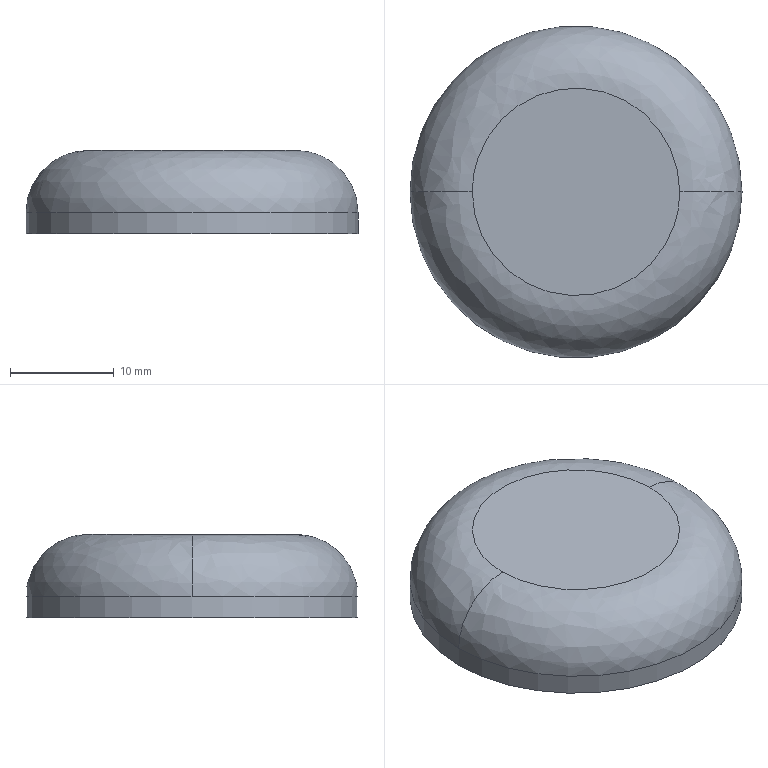Part | STEP file | 5091207W | 1 solid | 5 faces | box 32 x 32 x 8 mm | volume 5722 mm3 | plane 2 | spline 2 | cylinder 1 | commonest cylinder face diameters 32 x1
STEP:
#1=CARTESIAN_POINT('',(0.,0.,0.));
#2=DIRECTION('',(0.,0.,1.));
#3=DIRECTION('',(1.,0.,0.));
#4=AXIS2_PLACEMENT_3D('',#1,#2,#3);
#5=CARTESIAN_POINT('',(16.,-88.,34.));
#6=VERTEX_POINT('',#5);
#7=CARTESIAN_POINT('',(0.,-88.,34.));
#8=DIRECTION('',(0.,0.,1.));
#9=DIRECTION('',(1.,0.,0.));
#10=AXIS2_PLACEMENT_3D('',#7,#8,#9);
#11=CIRCLE('',#10,16.);
#12=CARTESIAN_POINT('',(16.64,-71.349,34.));
#13=DIRECTION('',(0.,0.,1.));
#14=DIRECTION('',(-1.,0.,0.));
#15=AXIS2_PLACEMENT_3D('',#12,#13,#14);
#16=PLANE('',#15);
#17=CARTESIAN_POINT('',(16.64,16.651));
#18=DIRECTION('',(-1.,0.));
#19=AXIS2_PLACEMENT_2D('',#17,#18);
#20=CIRCLE('',#19,16.);
#21=(GEOMETRIC_REPRESENTATION_CONTEXT(2)PARAMETRIC_REPRESENTATION_CONTEXT()REPRESENTATION_CONTEXT('',''));
#22=DEFINITIONAL_REPRESENTATION('',(#20),#21);
#23=PCURVE('',#16,#22);
#24=CARTESIAN_POINT('',(0.,-88.,34.));
#25=DIRECTION('',(0.,0.,1.));
#26=DIRECTION('',(1.,0.,0.));
#27=AXIS2_PLACEMENT_3D('',#24,#25,#26);
#28=CYLINDRICAL_SURFACE('',#27,16.);
#29=CARTESIAN_POINT('',(0.,0.));
#30=DIRECTION('',(1.,0.));
#31=VECTOR('',#30,1.);
#32=LINE('',#29,#31);
#33=(GEOMETRIC_REPRESENTATION_CONTEXT(2)PARAMETRIC_REPRESENTATION_CONTEXT()REPRESENTATION_CONTEXT('',''));
#34=DEFINITIONAL_REPRESENTATION('',(#32),#33);
#35=PCURVE('',#28,#34);
#36=SURFACE_CURVE('',#11,(#23,#35),.PCURVE_S1.);
#37=EDGE_CURVE('',#6,#6,#36,.T.);
#38=ORIENTED_EDGE('',*,*,#37,.F.);
#39=EDGE_LOOP('',(#38));
#40=FACE_BOUND('',#39,.T.);
#41=ADVANCED_FACE('',(#40),#16,.F.);
#42=ORIENTED_EDGE('',*,*,#37,.T.);
#43=CARTESIAN_POINT('',(16.,-88.,36.));
#44=VERTEX_POINT('',#43);
#45=CARTESIAN_POINT('',(16.,-88.,34.));
#46=CARTESIAN_POINT('',(16.,-88.,36.));
#47=B_SPLINE_CURVE_WITH_KNOTS('',1,(#45,#46),.UNSPECIFIED.,.F.,.F.,(2,2),(0.,2.),.PIECEWISE_BEZIER_KNOTS.);
#48=CARTESIAN_POINT('',(6.283,0.));
#49=DIRECTION('',(0.,1.));
#50=VECTOR('',#49,1.);
#51=LINE('',#48,#50);
#52=(GEOMETRIC_REPRESENTATION_CONTEXT(2)PARAMETRIC_REPRESENTATION_CONTEXT()REPRESENTATION_CONTEXT('',''));
#53=DEFINITIONAL_REPRESENTATION('',(#51),#52);
#54=PCURVE('',#28,#53);
#55=CARTESIAN_POINT('',(0.,0.));
#56=DIRECTION('',(0.,1.));
#57=VECTOR('',#56,1.);
#58=LINE('',#55,#57);
#59=(GEOMETRIC_REPRESENTATION_CONTEXT(2)PARAMETRIC_REPRESENTATION_CONTEXT()REPRESENTATION_CONTEXT('',''));
#60=DEFINITIONAL_REPRESENTATION('',(#58),#59);
#61=PCURVE('',#28,#60);
#62=SEAM_CURVE('',#47,(#54,#61),.PCURVE_S1.);
#63=EDGE_CURVE('',#6,#44,#62,.T.);
#64=ORIENTED_EDGE('',*,*,#63,.T.);
#65=CARTESIAN_POINT('',(-16.,-88.,36.));
#66=VERTEX_POINT('',#65);
#67=CARTESIAN_POINT('',(0.,-88.,36.));
#68=DIRECTION('',(0.,0.,1.));
#69=DIRECTION('',(-1.,0.,0.));
#70=AXIS2_PLACEMENT_3D('',#67,#68,#69);
#71=CIRCLE('',#70,16.);
#72=CARTESIAN_POINT('',(3.142,2.));
#73=DIRECTION('',(1.,0.));
#74=VECTOR('',#73,1.);
#75=LINE('',#72,#74);
#76=(GEOMETRIC_REPRESENTATION_CONTEXT(2)PARAMETRIC_REPRESENTATION_CONTEXT()REPRESENTATION_CONTEXT('',''));
#77=DEFINITIONAL_REPRESENTATION('',(#75),#76);
#78=PCURVE('',#28,#77);
#79=CARTESIAN_POINT('',(-16.,-88.,36.));
#80=CARTESIAN_POINT('',(-16.,-120.,36.));
#81=CARTESIAN_POINT('',(16.,-120.,36.));
#82=CARTESIAN_POINT('',(16.,-88.,36.));
#83=CARTESIAN_POINT('',(-16.,-88.,39.541));
#84=CARTESIAN_POINT('',(-16.,-120.,39.541));
#85=CARTESIAN_POINT('',(16.,-120.,39.541));
#86=CARTESIAN_POINT('',(16.,-88.,39.541));
#87=CARTESIAN_POINT('',(-13.485,-88.,42.03));
#88=CARTESIAN_POINT('',(-13.485,-114.97,42.03));
#89=CARTESIAN_POINT('',(13.485,-114.97,42.03));
#90=CARTESIAN_POINT('',(13.485,-88.,42.03));
#91=CARTESIAN_POINT('',(-9.949,-88.,42.));
#92=CARTESIAN_POINT('',(-9.949,-107.898,42.));
#93=CARTESIAN_POINT('',(9.949,-107.898,42.));
#94=CARTESIAN_POINT('',(9.949,-88.,42.));
#95=(BOUNDED_SURFACE()B_SPLINE_SURFACE(3,3,((#79,#80,#81,#82),(#83,#84,#85,#86),(#87,#88,#89,#90),(#91,#92,#93,#94)),.UNSPECIFIED.,.F.,.F.,.F.)B_SPLINE_SURFACE_WITH_KNOTS((4,4),(4,4),(0.0214,0.9843),(0.,1.),.PIECEWISE_BEZIER_KNOTS.)GEOMETRIC_REPRESENTATION_ITEM()RATIONAL_B_SPLINE_SURFACE(((0.9868,0.3289,0.3289,0.9868),(0.7929,0.2643,0.2643,0.7929),(0.7941,0.2647,0.2647,0.7941),(0.9903,0.3301,0.3301,0.9903)))REPRESENTATION_ITEM('')SURFACE());
#96=CARTESIAN_POINT('',(0.0214,0.));
#97=CARTESIAN_POINT('',(0.0214,0.02375));
#98=CARTESIAN_POINT('',(0.0214,0.06805));
#99=CARTESIAN_POINT('',(0.0214,0.1267));
#100=CARTESIAN_POINT('',(0.0214,0.1794));
#101=CARTESIAN_POINT('',(0.0214,0.2276));
#102=CARTESIAN_POINT('',(0.0214,0.2721));
#103=CARTESIAN_POINT('',(0.0214,0.3139));
#104=CARTESIAN_POINT('',(0.0214,0.3535));
#105=CARTESIAN_POINT('',(0.0214,0.3914));
#106=CARTESIAN_POINT('',(0.0214,0.4282));
#107=CARTESIAN_POINT('',(0.0214,0.4643));
#108=CARTESIAN_POINT('',(0.0214,0.5));
#109=CARTESIAN_POINT('',(0.0214,0.5357));
#110=CARTESIAN_POINT('',(0.0214,0.5718));
#111=CARTESIAN_POINT('',(0.0214,0.6086));
#112=CARTESIAN_POINT('',(0.0214,0.6465));
#113=CARTESIAN_POINT('',(0.0214,0.6861));
#114=CARTESIAN_POINT('',(0.0214,0.7279));
#115=CARTESIAN_POINT('',(0.0214,0.7724));
#116=CARTESIAN_POINT('',(0.0214,0.8206));
#117=CARTESIAN_POINT('',(0.0214,0.8733));
#118=CARTESIAN_POINT('',(0.0214,0.9319));
#119=CARTESIAN_POINT('',(0.0214,0.9763));
#120=CARTESIAN_POINT('',(0.0214,1.));
#121=B_SPLINE_CURVE_WITH_KNOTS('',3,(#96,#97,#98,#99,#100,#101,#102,#103,#104,#105,#106,#107,#108,#109,#110,#111,#112,#113,#114,#115,#116,#117,#118,#119,#120),.UNSPECIFIED.,.F.,.F.,(4,1,1,1,1,1,1,1,1,1,1,1,1,1,1,1,1,1,1,1,1,1,4),(0.,0.1428,0.2856,0.4284,0.5712,0.714,0.8568,0.9996,1.142,1.285,1.428,1.571,1.714,1.856,1.999,2.142,2.285,2.428,2.57,2.713,2.856,2.999,3.142),.QUASI_UNIFORM_KNOTS.);
#122=(GEOMETRIC_REPRESENTATION_CONTEXT(2)PARAMETRIC_REPRESENTATION_CONTEXT()REPRESENTATION_CONTEXT('',''));
#123=DEFINITIONAL_REPRESENTATION('',(#121),#122);
#124=PCURVE('',#95,#123);
#125=SURFACE_CURVE('',#71,(#78,#124),.PCURVE_S1.);
#126=EDGE_CURVE('',#66,#44,#125,.T.);
#127=ORIENTED_EDGE('',*,*,#126,.F.);
#128=CARTESIAN_POINT('',(0.,-88.,36.));
#129=DIRECTION('',(0.,0.,1.));
#130=DIRECTION('',(-1.,0.,0.));
#131=AXIS2_PLACEMENT_3D('',#128,#129,#130);
#132=CIRCLE('',#131,16.);
#133=CARTESIAN_POINT('',(-3.142,2.));
#134=DIRECTION('',(1.,0.));
#135=VECTOR('',#134,1.);
#136=LINE('',#133,#135);
#137=(GEOMETRIC_REPRESENTATION_CONTEXT(2)PARAMETRIC_REPRESENTATION_CONTEXT()REPRESENTATION_CONTEXT('',''));
#138=DEFINITIONAL_REPRESENTATION('',(#136),#137);
#139=PCURVE('',#28,#138);
#140=CARTESIAN_POINT('',(16.,-88.,36.));
#141=CARTESIAN_POINT('',(16.,-56.,36.));
#142=CARTESIAN_POINT('',(-16.,-56.,36.));
#143=CARTESIAN_POINT('',(-16.,-88.,36.));
#144=CARTESIAN_POINT('',(16.,-88.,39.541));
#145=CARTESIAN_POINT('',(16.,-56.,39.541));
#146=CARTESIAN_POINT('',(-16.,-56.,39.541));
#147=CARTESIAN_POINT('',(-16.,-88.,39.541));
#148=CARTESIAN_POINT('',(13.485,-88.,42.03));
#149=CARTESIAN_POINT('',(13.485,-61.03,42.03));
#150=CARTESIAN_POINT('',(-13.485,-61.03,42.03));
#151=CARTESIAN_POINT('',(-13.485,-88.,42.03));
#152=CARTESIAN_POINT('',(9.949,-88.,42.));
#153=CARTESIAN_POINT('',(9.949,-68.102,42.));
#154=CARTESIAN_POINT('',(-9.949,-68.102,42.));
#155=CARTESIAN_POINT('',(-9.949,-88.,42.));
#156=(BOUNDED_SURFACE()B_SPLINE_SURFACE(3,3,((#140,#141,#142,#143),(#144,#145,#146,#147),(#148,#149,#150,#151),(#152,#153,#154,#155)),.UNSPECIFIED.,.F.,.F.,.F.)B_SPLINE_SURFACE_WITH_KNOTS((4,4),(4,4),(0.0214,0.9843),(0.,1.),.PIECEWISE_BEZIER_KNOTS.)GEOMETRIC_REPRESENTATION_ITEM()RATIONAL_B_SPLINE_SURFACE(((0.9868,0.3289,0.3289,0.9868),(0.7929,0.2643,0.2643,0.7929),(0.7941,0.2647,0.2647,0.7941),(0.9903,0.3301,0.3301,0.9903)))REPRESENTATION_ITEM('')SURFACE());
#157=CARTESIAN_POINT('',(0.0214,0.));
#158=CARTESIAN_POINT('',(0.0214,0.02375));
#159=CARTESIAN_POINT('',(0.0214,0.06805));
#160=CARTESIAN_POINT('',(0.0214,0.1267));
#161=CARTESIAN_POINT('',(0.0214,0.1794));
#162=CARTESIAN_POINT('',(0.0214,0.2276));
#163=CARTESIAN_POINT('',(0.0214,0.2721));
#164=CARTESIAN_POINT('',(0.0214,0.3139));
#165=CARTESIAN_POINT('',(0.0214,0.3535));
#166=CARTESIAN_POINT('',(0.0214,0.3914));
#167=CARTESIAN_POINT('',(0.0214,0.4282));
#168=CARTESIAN_POINT('',(0.0214,0.4643));
#169=CARTESIAN_POINT('',(0.0214,0.5));
#170=CARTESIAN_POINT('',(0.0214,0.5357));
#171=CARTESIAN_POINT('',(0.0214,0.5718));
#172=CARTESIAN_POINT('',(0.0214,0.6086));
#173=CARTESIAN_POINT('',(0.0214,0.6465));
#174=CARTESIAN_POINT('',(0.0214,0.6861));
#175=CARTESIAN_POINT('',(0.0214,0.7279));
#176=CARTESIAN_POINT('',(0.0214,0.7724));
#177=CARTESIAN_POINT('',(0.0214,0.8206));
#178=CARTESIAN_POINT('',(0.0214,0.8733));
#179=CARTESIAN_POINT('',(0.0214,0.9319));
#180=CARTESIAN_POINT('',(0.0214,0.9763));
#181=CARTESIAN_POINT('',(0.0214,1.));
#182=B_SPLINE_CURVE_WITH_KNOTS('',3,(#157,#158,#159,#160,#161,#162,#163,#164,#165,#166,#167,#168,#169,#170,#171,#172,#173,#174,#175,#176,#177,#178,#179,#180,#181),.UNSPECIFIED.,.F.,.F.,(4,1,1,1,1,1,1,1,1,1,1,1,1,1,1,1,1,1,1,1,1,1,4),(3.142,3.284,3.427,3.57,3.713,3.856,3.998,4.141,4.284,4.427,4.57,4.712,4.855,4.998,5.141,5.284,5.426,5.569,5.712,5.855,5.998,6.14,6.283),.QUASI_UNIFORM_KNOTS.);
#183=(GEOMETRIC_REPRESENTATION_CONTEXT(2)PARAMETRIC_REPRESENTATION_CONTEXT()REPRESENTATION_CONTEXT('',''));
#184=DEFINITIONAL_REPRESENTATION('',(#182),#183);
#185=PCURVE('',#156,#184);
#186=SURFACE_CURVE('',#132,(#139,#185),.PCURVE_S1.);
#187=EDGE_CURVE('',#44,#66,#186,.T.);
#188=ORIENTED_EDGE('',*,*,#187,.F.);
#189=ORIENTED_EDGE('',*,*,#63,.F.);
#190=EDGE_LOOP('',(#42,#64,#127,#188,#189));
#191=FACE_BOUND('',#190,.T.);
#192=ADVANCED_FACE('',(#191),#28,.T.);
#193=CARTESIAN_POINT('',(10.,-88.,42.));
#194=VERTEX_POINT('',#193);
#195=CARTESIAN_POINT('',(10.,-88.,36.));
#196=DIRECTION('',(0.,-1.,0.));
#197=DIRECTION('',(1.,0.,0.));
#198=AXIS2_PLACEMENT_3D('',#195,#196,#197);
#199=CIRCLE('',#198,6.);
#200=CARTESIAN_POINT('',(0.0214,0.));
#201=CARTESIAN_POINT('',(0.03751,0.));
#202=CARTESIAN_POINT('',(0.06926,0.));
#203=CARTESIAN_POINT('',(0.1156,0.));
#204=CARTESIAN_POINT('',(0.1609,0.));
#205=CARTESIAN_POINT('',(0.2052,0.));
#206=CARTESIAN_POINT('',(0.2488,0.));
#207=CARTESIAN_POINT('',(0.2916,0.));
#208=CARTESIAN_POINT('',(0.3339,0.));
#209=CARTESIAN_POINT('',(0.3758,0.));
#210=CARTESIAN_POINT('',(0.4174,0.));
#211=CARTESIAN_POINT('',(0.4588,0.));
#212=CARTESIAN_POINT('',(0.5,0.));
#213=CARTESIAN_POINT('',(0.5412,0.));
#214=CARTESIAN_POINT('',(0.5826,0.));
#215=CARTESIAN_POINT('',(0.6242,0.));
#216=CARTESIAN_POINT('',(0.6661,0.));
#217=CARTESIAN_POINT('',(0.7084,0.));
#218=CARTESIAN_POINT('',(0.7512,0.));
#219=CARTESIAN_POINT('',(0.7948,0.));
#220=CARTESIAN_POINT('',(0.8391,0.));
#221=CARTESIAN_POINT('',(0.8844,0.));
#222=CARTESIAN_POINT('',(0.9307,0.));
#223=CARTESIAN_POINT('',(0.9625,0.));
#224=CARTESIAN_POINT('',(0.9786,0.));
#225=B_SPLINE_CURVE_WITH_KNOTS('',3,(#200,#201,#202,#203,#204,#205,#206,#207,#208,#209,#210,#211,#212,#213,#214,#215,#216,#217,#218,#219,#220,#221,#222,#223,#224),.UNSPECIFIED.,.F.,.F.,(4,1,1,1,1,1,1,1,1,1,1,1,1,1,1,1,1,1,1,1,1,1,4),(0.,0.0714,0.1428,0.2142,0.2856,0.357,0.4284,0.4998,0.5712,0.6426,0.714,0.7854,0.8568,0.9282,0.9996,1.071,1.142,1.214,1.285,1.357,1.428,1.499,1.571),.QUASI_UNIFORM_KNOTS.);
#226=(GEOMETRIC_REPRESENTATION_CONTEXT(2)PARAMETRIC_REPRESENTATION_CONTEXT()REPRESENTATION_CONTEXT('',''));
#227=DEFINITIONAL_REPRESENTATION('',(#225),#226);
#228=PCURVE('',#156,#227);
#229=CARTESIAN_POINT('',(0.0214,1.));
#230=CARTESIAN_POINT('',(0.03751,1.));
#231=CARTESIAN_POINT('',(0.06926,1.));
#232=CARTESIAN_POINT('',(0.1156,1.));
#233=CARTESIAN_POINT('',(0.1609,1.));
#234=CARTESIAN_POINT('',(0.2052,1.));
#235=CARTESIAN_POINT('',(0.2488,1.));
#236=CARTESIAN_POINT('',(0.2916,1.));
#237=CARTESIAN_POINT('',(0.3339,1.));
#238=CARTESIAN_POINT('',(0.3758,1.));
#239=CARTESIAN_POINT('',(0.4174,1.));
#240=CARTESIAN_POINT('',(0.4588,1.));
#241=CARTESIAN_POINT('',(0.5,1.));
#242=CARTESIAN_POINT('',(0.5412,1.));
#243=CARTESIAN_POINT('',(0.5826,1.));
#244=CARTESIAN_POINT('',(0.6242,1.));
#245=CARTESIAN_POINT('',(0.6661,1.));
#246=CARTESIAN_POINT('',(0.7084,1.));
#247=CARTESIAN_POINT('',(0.7512,1.));
#248=CARTESIAN_POINT('',(0.7948,1.));
#249=CARTESIAN_POINT('',(0.8391,1.));
#250=CARTESIAN_POINT('',(0.8844,1.));
#251=CARTESIAN_POINT('',(0.9307,1.));
#252=CARTESIAN_POINT('',(0.9625,1.));
#253=CARTESIAN_POINT('',(0.9786,1.));
#254=B_SPLINE_CURVE_WITH_KNOTS('',3,(#229,#230,#231,#232,#233,#234,#235,#236,#237,#238,#239,#240,#241,#242,#243,#244,#245,#246,#247,#248,#249,#250,#251,#252,#253),.UNSPECIFIED.,.F.,.F.,(4,1,1,1,1,1,1,1,1,1,1,1,1,1,1,1,1,1,1,1,1,1,4),(0.,0.0714,0.1428,0.2142,0.2856,0.357,0.4284,0.4998,0.5712,0.6426,0.714,0.7854,0.8568,0.9282,0.9996,1.071,1.142,1.214,1.285,1.357,1.428,1.499,1.571),.QUASI_UNIFORM_KNOTS.);
#255=(GEOMETRIC_REPRESENTATION_CONTEXT(2)PARAMETRIC_REPRESENTATION_CONTEXT()REPRESENTATION_CONTEXT('',''));
#256=DEFINITIONAL_REPRESENTATION('',(#254),#255);
#257=PCURVE('',#95,#256);
#258=SURFACE_CURVE('',#199,(#228,#257),.PCURVE_S1.);
#259=EDGE_CURVE('',#44,#194,#258,.T.);
#260=ORIENTED_EDGE('',*,*,#259,.T.);
#261=CARTESIAN_POINT('',(-10.,-87.956,42.));
#262=VERTEX_POINT('',#261);
#263=CARTESIAN_POINT('',(10.,-88.,42.));
#264=CARTESIAN_POINT('',(10.,-87.344,42.));
#265=CARTESIAN_POINT('',(9.936,-86.695,42.));
#266=CARTESIAN_POINT('',(9.681,-85.409,42.));
#267=CARTESIAN_POINT('',(9.491,-84.784,42.));
#268=CARTESIAN_POINT('',(8.99,-83.573,42.));
#269=CARTESIAN_POINT('',(8.683,-82.996,42.));
#270=CARTESIAN_POINT('',(7.956,-81.906,42.));
#271=CARTESIAN_POINT('',(7.542,-81.401,42.));
#272=CARTESIAN_POINT('',(6.616,-80.473,42.));
#273=CARTESIAN_POINT('',(6.112,-80.058,42.));
#274=CARTESIAN_POINT('',(5.023,-79.328,42.));
#275=CARTESIAN_POINT('',(4.447,-79.019,42.));
#276=CARTESIAN_POINT('',(3.237,-78.516,42.));
#277=CARTESIAN_POINT('',(2.612,-78.325,42.));
#278=CARTESIAN_POINT('',(1.327,-78.067,42.));
#279=CARTESIAN_POINT('',(0.6774,-78.002,42.));
#280=CARTESIAN_POINT('',(-0.6332,-77.999,42.));
#281=CARTESIAN_POINT('',(-1.283,-78.061,42.));
#282=CARTESIAN_POINT('',(-2.57,-78.314,42.));
#283=CARTESIAN_POINT('',(-3.195,-78.502,42.));
#284=CARTESIAN_POINT('',(-4.407,-79.,42.));
#285=CARTESIAN_POINT('',(-4.984,-79.306,42.));
#286=CARTESIAN_POINT('',(-6.076,-80.031,42.));
#287=CARTESIAN_POINT('',(-6.583,-80.444,42.));
#288=CARTESIAN_POINT('',(-7.513,-81.367,42.));
#289=CARTESIAN_POINT('',(-7.929,-81.871,42.));
#290=CARTESIAN_POINT('',(-8.661,-82.958,42.));
#291=CARTESIAN_POINT('',(-8.971,-83.533,42.));
#292=CARTESIAN_POINT('',(-9.477,-84.742,42.));
#293=CARTESIAN_POINT('',(-9.669,-85.367,42.));
#294=CARTESIAN_POINT('',(-9.93,-86.651,42.));
#295=CARTESIAN_POINT('',(-9.997,-87.3,42.));
#296=CARTESIAN_POINT('',(-10.,-87.956,42.));
#297=B_SPLINE_CURVE_WITH_KNOTS('',3,(#263,#264,#265,#266,#267,#268,#269,#270,#271,#272,#273,#274,#275,#276,#277,#278,#279,#280,#281,#282,#283,#284,#285,#286,#287,#288,#289,#290,#291,#292,#293,#294,#295,#296),.UNSPECIFIED.,.F.,.F.,(4,2,2,2,2,2,2,2,2,2,2,2,2,2,2,2,4),(0.,0.0625,0.125,0.1875,0.25,0.3125,0.375,0.4375,0.5,0.5625,0.625,0.6875,0.75,0.8125,0.875,0.9375,1.),.UNSPECIFIED.);
#298=CARTESIAN_POINT('',(0.9786,0.));
#299=CARTESIAN_POINT('',(0.9786,0.007948));
#300=CARTESIAN_POINT('',(0.9786,0.02343));
#301=CARTESIAN_POINT('',(0.9786,0.04558));
#302=CARTESIAN_POINT('',(0.9786,0.06678));
#303=CARTESIAN_POINT('',(0.9786,0.08717));
#304=CARTESIAN_POINT('',(0.9786,0.1068));
#305=CARTESIAN_POINT('',(0.9786,0.1257));
#306=CARTESIAN_POINT('',(0.9786,0.1439));
#307=CARTESIAN_POINT('',(0.9786,0.1615));
#308=CARTESIAN_POINT('',(0.9786,0.1786));
#309=CARTESIAN_POINT('',(0.9786,0.1951));
#310=CARTESIAN_POINT('',(0.9786,0.2111));
#311=CARTESIAN_POINT('',(0.9786,0.2268));
#312=CARTESIAN_POINT('',(0.9786,0.242));
#313=CARTESIAN_POINT('',(0.9786,0.2569));
#314=CARTESIAN_POINT('',(0.9786,0.2714));
#315=CARTESIAN_POINT('',(0.9786,0.2856));
#316=CARTESIAN_POINT('',(0.9786,0.2996));
#317=CARTESIAN_POINT('',(0.9786,0.3132));
#318=CARTESIAN_POINT('',(0.9786,0.3266));
#319=CARTESIAN_POINT('',(0.9786,0.3398));
#320=CARTESIAN_POINT('',(0.9786,0.3529));
#321=CARTESIAN_POINT('',(0.9786,0.3657));
#322=CARTESIAN_POINT('',(0.9786,0.3783));
#323=CARTESIAN_POINT('',(0.9786,0.3908));
#324=CARTESIAN_POINT('',(0.9786,0.4032));
#325=CARTESIAN_POINT('',(0.9786,0.4155));
#326=CARTESIAN_POINT('',(0.9786,0.4277));
#327=CARTESIAN_POINT('',(0.9786,0.4397));
#328=CARTESIAN_POINT('',(0.9786,0.4518));
#329=CARTESIAN_POINT('',(0.9786,0.4638));
#330=CARTESIAN_POINT('',(0.9786,0.4757));
#331=CARTESIAN_POINT('',(0.9786,0.4875));
#332=CARTESIAN_POINT('',(0.9786,0.4994));
#333=CARTESIAN_POINT('',(0.9786,0.5113));
#334=CARTESIAN_POINT('',(0.9786,0.5232));
#335=CARTESIAN_POINT('',(0.9786,0.5351));
#336=CARTESIAN_POINT('',(0.9786,0.5471));
#337=CARTESIAN_POINT('',(0.9786,0.5591));
#338=CARTESIAN_POINT('',(0.9786,0.5712));
#339=CARTESIAN_POINT('',(0.9786,0.5834));
#340=CARTESIAN_POINT('',(0.9786,0.5956));
#341=CARTESIAN_POINT('',(0.9786,0.608));
#342=CARTESIAN_POINT('',(0.9786,0.6205));
#343=CARTESIAN_POINT('',(0.9786,0.6331));
#344=CARTESIAN_POINT('',(0.9786,0.6459));
#345=CARTESIAN_POINT('',(0.9786,0.659));
#346=CARTESIAN_POINT('',(0.9786,0.6721));
#347=CARTESIAN_POINT('',(0.9786,0.6855));
#348=CARTESIAN_POINT('',(0.9786,0.6992));
#349=CARTESIAN_POINT('',(0.9786,0.7131));
#350=CARTESIAN_POINT('',(0.9786,0.7273));
#351=CARTESIAN_POINT('',(0.9786,0.7417));
#352=CARTESIAN_POINT('',(0.9786,0.7566));
#353=CARTESIAN_POINT('',(0.9786,0.7718));
#354=CARTESIAN_POINT('',(0.9786,0.7874));
#355=CARTESIAN_POINT('',(0.9786,0.8034));
#356=CARTESIAN_POINT('',(0.9786,0.8199));
#357=CARTESIAN_POINT('',(0.9786,0.8369));
#358=CARTESIAN_POINT('',(0.9786,0.8545));
#359=CARTESIAN_POINT('',(0.9786,0.8726));
#360=CARTESIAN_POINT('',(0.9786,0.8914));
#361=CARTESIAN_POINT('',(0.9786,0.911));
#362=CARTESIAN_POINT('',(0.9786,0.9313));
#363=CARTESIAN_POINT('',(0.9786,0.9524));
#364=CARTESIAN_POINT('',(0.9786,0.9745));
#365=CARTESIAN_POINT('',(0.9786,0.9899));
#366=CARTESIAN_POINT('',(0.9786,0.9978));
#367=B_SPLINE_CURVE_WITH_KNOTS('',3,(#298,#299,#300,#301,#302,#303,#304,#305,#306,#307,#308,#309,#310,#311,#312,#313,#314,#315,#316,#317,#318,#319,#320,#321,#322,#323,#324,#325,#326,#327,#328,#329,#330,#331,#332,#333,#334,#335,#336,#337,#338,#339,#340,#341,#342,#343,#344,#345,#346,#347,#348,#349,#350,#351,#352,#353,#354,#355,#356,#357,#358,#359,#360,#361,#362,#363,#364,#365,#366),.UNSPECIFIED.,.F.,.F.,(4,1,1,1,1,1,1,1,1,1,1,1,1,1,1,1,1,1,1,1,1,1,1,1,1,1,1,1,1,1,1,1,1,1,1,1,1,1,1,1,1,1,1,1,1,1,1,1,1,1,1,1,1,1,1,1,1,1,1,1,1,1,1,1,1,1,4),(0.,0.01515,0.0303,0.04545,0.06061,0.07576,0.09091,0.1061,0.1212,0.1364,0.1515,0.1667,0.1818,0.197,0.2121,0.2273,0.2424,0.2576,0.2727,0.2879,0.303,0.3182,0.3333,0.3485,0.3636,0.3788,0.3939,0.4091,0.4242,0.4394,0.4545,0.4697,0.4848,0.5,0.5152,0.5303,0.5455,0.5606,0.5758,0.5909,0.6061,0.6212,0.6364,0.6515,0.6667,0.6818,0.697,0.7121,0.7273,0.7424,0.7576,0.7727,0.7879,0.803,0.8182,0.8333,0.8485,0.8636,0.8788,0.8939,0.9091,0.9242,0.9394,0.9545,0.9697,0.9848,1.),.QUASI_UNIFORM_KNOTS.);
#368=(GEOMETRIC_REPRESENTATION_CONTEXT(2)PARAMETRIC_REPRESENTATION_CONTEXT()REPRESENTATION_CONTEXT('',''));
#369=DEFINITIONAL_REPRESENTATION('',(#367),#368);
#370=PCURVE('',#156,#369);
#371=CARTESIAN_POINT('',(10.4,-77.592,42.));
#372=DIRECTION('',(0.,0.,1.));
#373=DIRECTION('',(-1.,0.,0.));
#374=AXIS2_PLACEMENT_3D('',#371,#372,#373);
#375=PLANE('',#374);
#376=CARTESIAN_POINT('',(0.4,10.408));
#377=CARTESIAN_POINT('',(0.4001,9.752));
#378=CARTESIAN_POINT('',(0.464,9.103));
#379=CARTESIAN_POINT('',(0.7192,7.817));
#380=CARTESIAN_POINT('',(0.9087,7.192));
#381=CARTESIAN_POINT('',(1.409,5.981));
#382=CARTESIAN_POINT('',(1.717,5.405));
#383=CARTESIAN_POINT('',(2.444,4.314));
#384=CARTESIAN_POINT('',(2.858,3.809));
#385=CARTESIAN_POINT('',(3.784,2.881));
#386=CARTESIAN_POINT('',(4.288,2.466));
#387=CARTESIAN_POINT('',(5.377,1.736));
#388=CARTESIAN_POINT('',(5.953,1.428));
#389=CARTESIAN_POINT('',(7.163,0.9239));
#390=CARTESIAN_POINT('',(7.788,0.7332));
#391=CARTESIAN_POINT('',(9.073,0.475));
#392=CARTESIAN_POINT('',(9.723,0.4096));
#393=CARTESIAN_POINT('',(11.033,0.4067));
#394=CARTESIAN_POINT('',(11.683,0.4693));
#395=CARTESIAN_POINT('',(12.97,0.7217));
#396=CARTESIAN_POINT('',(13.595,0.9097));
#397=CARTESIAN_POINT('',(14.807,1.408));
#398=CARTESIAN_POINT('',(15.384,1.714));
#399=CARTESIAN_POINT('',(16.476,2.439));
#400=CARTESIAN_POINT('',(16.983,2.852));
#401=CARTESIAN_POINT('',(17.913,3.776));
#402=CARTESIAN_POINT('',(18.329,4.279));
#403=CARTESIAN_POINT('',(19.061,5.366));
#404=CARTESIAN_POINT('',(19.371,5.941));
#405=CARTESIAN_POINT('',(19.877,7.15));
#406=CARTESIAN_POINT('',(20.069,7.775));
#407=CARTESIAN_POINT('',(20.33,9.059));
#408=CARTESIAN_POINT('',(20.397,9.708));
#409=CARTESIAN_POINT('',(20.4,10.364));
#410=B_SPLINE_CURVE_WITH_KNOTS('',3,(#376,#377,#378,#379,#380,#381,#382,#383,#384,#385,#386,#387,#388,#389,#390,#391,#392,#393,#394,#395,#396,#397,#398,#399,#400,#401,#402,#403,#404,#405,#406,#407,#408,#409),.UNSPECIFIED.,.F.,.F.,(4,2,2,2,2,2,2,2,2,2,2,2,2,2,2,2,4),(0.,0.0625,0.125,0.1875,0.25,0.3125,0.375,0.4375,0.5,0.5625,0.625,0.6875,0.75,0.8125,0.875,0.9375,1.),.UNSPECIFIED.);
#411=(GEOMETRIC_REPRESENTATION_CONTEXT(2)PARAMETRIC_REPRESENTATION_CONTEXT()REPRESENTATION_CONTEXT('',''));
#412=DEFINITIONAL_REPRESENTATION('',(#410),#411);
#413=PCURVE('',#375,#412);
#414=SURFACE_CURVE('',#297,(#370,#413),.PCURVE_S1.);
#415=EDGE_CURVE('',#194,#262,#414,.T.);
#416=ORIENTED_EDGE('',*,*,#415,.T.);
#417=CARTESIAN_POINT('',(-10.,-88.,42.));
#418=VERTEX_POINT('',#417);
#419=CARTESIAN_POINT('',(-10.,-87.956,42.));
#420=DIRECTION('',(0.002208,1.,0.));
#421=VECTOR('',#420,1.);
#422=LINE('',#419,#421);
#423=CARTESIAN_POINT('',(0.9786,1.));
#424=CARTESIAN_POINT('',(0.9786,1.));
#425=CARTESIAN_POINT('',(0.9786,0.9999));
#426=CARTESIAN_POINT('',(0.9786,0.9998));
#427=CARTESIAN_POINT('',(0.9786,0.9997));
#428=CARTESIAN_POINT('',(0.9786,0.9996));
#429=CARTESIAN_POINT('',(0.9786,0.9995));
#430=CARTESIAN_POINT('',(0.9786,0.9994));
#431=CARTESIAN_POINT('',(0.9786,0.9993));
#432=CARTESIAN_POINT('',(0.9786,0.9992));
#433=CARTESIAN_POINT('',(0.9786,0.9991));
#434=CARTESIAN_POINT('',(0.9786,0.999));
#435=CARTESIAN_POINT('',(0.9786,0.9989));
#436=CARTESIAN_POINT('',(0.9786,0.9988));
#437=CARTESIAN_POINT('',(0.9786,0.9987));
#438=CARTESIAN_POINT('',(0.9786,0.9986));
#439=CARTESIAN_POINT('',(0.9786,0.9985));
#440=CARTESIAN_POINT('',(0.9786,0.9984));
#441=CARTESIAN_POINT('',(0.9786,0.9983));
#442=CARTESIAN_POINT('',(0.9786,0.9982));
#443=CARTESIAN_POINT('',(0.9786,0.9981));
#444=CARTESIAN_POINT('',(0.9786,0.998));
#445=CARTESIAN_POINT('',(0.9786,0.9979));
#446=CARTESIAN_POINT('',(0.9786,0.9978));
#447=CARTESIAN_POINT('',(0.9786,0.9978));
#448=B_SPLINE_CURVE_WITH_KNOTS('',3,(#423,#424,#425,#426,#427,#428,#429,#430,#431,#432,#433,#434,#435,#436,#437,#438,#439,#440,#441,#442,#443,#444,#445,#446,#447),.UNSPECIFIED.,.F.,.F.,(4,1,1,1,1,1,1,1,1,1,1,1,1,1,1,1,1,1,1,1,1,1,4),(-0.04416,-0.04216,-0.04015,-0.03814,-0.03613,-0.03413,-0.03212,-0.03011,-0.0281,-0.0261,-0.02409,-0.02208,-0.02007,-0.01807,-0.01606,-0.01405,-0.01204,-0.01004,-0.00803,-0.006022,-0.004015,-0.002007,0.),.UNSPECIFIED.);
#449=(GEOMETRIC_REPRESENTATION_CONTEXT(2)PARAMETRIC_REPRESENTATION_CONTEXT()REPRESENTATION_CONTEXT('',''));
#450=DEFINITIONAL_REPRESENTATION('',(#448),#449);
#451=PCURVE('',#156,#450);
#452=CARTESIAN_POINT('',(20.4,10.364));
#453=DIRECTION('',(-0.002208,-1.));
#454=VECTOR('',#453,1.);
#455=LINE('',#452,#454);
#456=(GEOMETRIC_REPRESENTATION_CONTEXT(2)PARAMETRIC_REPRESENTATION_CONTEXT()REPRESENTATION_CONTEXT('',''));
#457=DEFINITIONAL_REPRESENTATION('',(#455),#456);
#458=PCURVE('',#375,#457);
#459=SURFACE_CURVE('',#422,(#451,#458),.PCURVE_S1.);
#460=EDGE_CURVE('',#418,#262,#459,.T.);
#461=ORIENTED_EDGE('',*,*,#460,.F.);
#462=CARTESIAN_POINT('',(-10.,-88.,36.));
#463=DIRECTION('',(0.,-1.,0.));
#464=DIRECTION('',(1.,0.,0.));
#465=AXIS2_PLACEMENT_3D('',#462,#463,#464);
#466=CIRCLE('',#465,6.);
#467=CARTESIAN_POINT('',(0.9786,1.));
#468=CARTESIAN_POINT('',(0.9625,1.));
#469=CARTESIAN_POINT('',(0.9307,1.));
#470=CARTESIAN_POINT('',(0.8844,1.));
#471=CARTESIAN_POINT('',(0.8391,1.));
#472=CARTESIAN_POINT('',(0.7948,1.));
#473=CARTESIAN_POINT('',(0.7512,1.));
#474=CARTESIAN_POINT('',(0.7084,1.));
#475=CARTESIAN_POINT('',(0.6661,1.));
#476=CARTESIAN_POINT('',(0.6242,1.));
#477=CARTESIAN_POINT('',(0.5826,1.));
#478=CARTESIAN_POINT('',(0.5412,1.));
#479=CARTESIAN_POINT('',(0.5,1.));
#480=CARTESIAN_POINT('',(0.4588,1.));
#481=CARTESIAN_POINT('',(0.4174,1.));
#482=CARTESIAN_POINT('',(0.3758,1.));
#483=CARTESIAN_POINT('',(0.3339,1.));
#484=CARTESIAN_POINT('',(0.2916,1.));
#485=CARTESIAN_POINT('',(0.2488,1.));
#486=CARTESIAN_POINT('',(0.2052,1.));
#487=CARTESIAN_POINT('',(0.1609,1.));
#488=CARTESIAN_POINT('',(0.1156,1.));
#489=CARTESIAN_POINT('',(0.06926,1.));
#490=CARTESIAN_POINT('',(0.03751,1.));
#491=CARTESIAN_POINT('',(0.0214,1.));
#492=B_SPLINE_CURVE_WITH_KNOTS('',3,(#467,#468,#469,#470,#471,#472,#473,#474,#475,#476,#477,#478,#479,#480,#481,#482,#483,#484,#485,#486,#487,#488,#489,#490,#491),.UNSPECIFIED.,.F.,.F.,(4,1,1,1,1,1,1,1,1,1,1,1,1,1,1,1,1,1,1,1,1,1,4),(1.571,1.642,1.714,1.785,1.856,1.928,1.999,2.071,2.142,2.213,2.285,2.356,2.428,2.499,2.57,2.642,2.713,2.785,2.856,2.927,2.999,3.07,3.142),.QUASI_UNIFORM_KNOTS.);
#493=(GEOMETRIC_REPRESENTATION_CONTEXT(2)PARAMETRIC_REPRESENTATION_CONTEXT()REPRESENTATION_CONTEXT('',''));
#494=DEFINITIONAL_REPRESENTATION('',(#492),#493);
#495=PCURVE('',#156,#494);
#496=CARTESIAN_POINT('',(0.9786,0.));
#497=CARTESIAN_POINT('',(0.9625,0.));
#498=CARTESIAN_POINT('',(0.9307,0.));
#499=CARTESIAN_POINT('',(0.8844,0.));
#500=CARTESIAN_POINT('',(0.8391,0.));
#501=CARTESIAN_POINT('',(0.7948,0.));
#502=CARTESIAN_POINT('',(0.7512,0.));
#503=CARTESIAN_POINT('',(0.7084,0.));
#504=CARTESIAN_POINT('',(0.6661,0.));
#505=CARTESIAN_POINT('',(0.6242,0.));
#506=CARTESIAN_POINT('',(0.5826,0.));
#507=CARTESIAN_POINT('',(0.5412,0.));
#508=CARTESIAN_POINT('',(0.5,0.));
#509=CARTESIAN_POINT('',(0.4588,0.));
#510=CARTESIAN_POINT('',(0.4174,0.));
#511=CARTESIAN_POINT('',(0.3758,0.));
#512=CARTESIAN_POINT('',(0.3339,0.));
#513=CARTESIAN_POINT('',(0.2916,0.));
#514=CARTESIAN_POINT('',(0.2488,0.));
#515=CARTESIAN_POINT('',(0.2052,0.));
#516=CARTESIAN_POINT('',(0.1609,0.));
#517=CARTESIAN_POINT('',(0.1156,0.));
#518=CARTESIAN_POINT('',(0.06926,0.));
#519=CARTESIAN_POINT('',(0.03751,0.));
#520=CARTESIAN_POINT('',(0.0214,0.));
#521=B_SPLINE_CURVE_WITH_KNOTS('',3,(#496,#497,#498,#499,#500,#501,#502,#503,#504,#505,#506,#507,#508,#509,#510,#511,#512,#513,#514,#515,#516,#517,#518,#519,#520),.UNSPECIFIED.,.F.,.F.,(4,1,1,1,1,1,1,1,1,1,1,1,1,1,1,1,1,1,1,1,1,1,4),(1.571,1.642,1.714,1.785,1.856,1.928,1.999,2.071,2.142,2.213,2.285,2.356,2.428,2.499,2.57,2.642,2.713,2.785,2.856,2.927,2.999,3.07,3.142),.QUASI_UNIFORM_KNOTS.);
#522=(GEOMETRIC_REPRESENTATION_CONTEXT(2)PARAMETRIC_REPRESENTATION_CONTEXT()REPRESENTATION_CONTEXT('',''));
#523=DEFINITIONAL_REPRESENTATION('',(#521),#522);
#524=PCURVE('',#95,#523);
#525=SURFACE_CURVE('',#466,(#495,#524),.PCURVE_S1.);
#526=EDGE_CURVE('',#418,#66,#525,.T.);
#527=ORIENTED_EDGE('',*,*,#526,.T.);
#528=ORIENTED_EDGE('',*,*,#187,.F.);
#529=EDGE_LOOP('',(#260,#416,#461,#527,#528));
#530=FACE_BOUND('',#529,.F.);
#531=ADVANCED_FACE('',(#530),#156,.F.);
#532=ORIENTED_EDGE('',*,*,#526,.F.);
#533=CARTESIAN_POINT('',(10.,-88.044,42.));
#534=VERTEX_POINT('',#533);
#535=CARTESIAN_POINT('',(-10.,-88.,42.));
#536=CARTESIAN_POINT('',(-10.,-88.656,42.));
#537=CARTESIAN_POINT('',(-9.936,-89.305,42.));
#538=CARTESIAN_POINT('',(-9.681,-90.591,42.));
#539=CARTESIAN_POINT('',(-9.491,-91.216,42.));
#540=CARTESIAN_POINT('',(-8.99,-92.427,42.));
#541=CARTESIAN_POINT('',(-8.683,-93.004,42.));
#542=CARTESIAN_POINT('',(-7.956,-94.094,42.));
#543=CARTESIAN_POINT('',(-7.542,-94.599,42.));
#544=CARTESIAN_POINT('',(-6.616,-95.527,42.));
#545=CARTESIAN_POINT('',(-6.112,-95.942,42.));
#546=CARTESIAN_POINT('',(-5.023,-96.672,42.));
#547=CARTESIAN_POINT('',(-4.447,-96.981,42.));
#548=CARTESIAN_POINT('',(-3.237,-97.484,42.));
#549=CARTESIAN_POINT('',(-2.612,-97.675,42.));
#550=CARTESIAN_POINT('',(-1.327,-97.933,42.));
#551=CARTESIAN_POINT('',(-0.6774,-97.998,42.));
#552=CARTESIAN_POINT('',(0.6332,-98.001,42.));
#553=CARTESIAN_POINT('',(1.283,-97.939,42.));
#554=CARTESIAN_POINT('',(2.57,-97.686,42.));
#555=CARTESIAN_POINT('',(3.195,-97.498,42.));
#556=CARTESIAN_POINT('',(4.407,-97.,42.));
#557=CARTESIAN_POINT('',(4.984,-96.694,42.));
#558=CARTESIAN_POINT('',(6.076,-95.969,42.));
#559=CARTESIAN_POINT('',(6.583,-95.556,42.));
#560=CARTESIAN_POINT('',(7.513,-94.633,42.));
#561=CARTESIAN_POINT('',(7.929,-94.129,42.));
#562=CARTESIAN_POINT('',(8.661,-93.042,42.));
#563=CARTESIAN_POINT('',(8.971,-92.467,42.));
#564=CARTESIAN_POINT('',(9.477,-91.258,42.));
#565=CARTESIAN_POINT('',(9.669,-90.633,42.));
#566=CARTESIAN_POINT('',(9.93,-89.349,42.));
#567=CARTESIAN_POINT('',(9.997,-88.7,42.));
#568=CARTESIAN_POINT('',(10.,-88.044,42.));
#569=B_SPLINE_CURVE_WITH_KNOTS('',3,(#535,#536,#537,#538,#539,#540,#541,#542,#543,#544,#545,#546,#547,#548,#549,#550,#551,#552,#553,#554,#555,#556,#557,#558,#559,#560,#561,#562,#563,#564,#565,#566,#567,#568),.UNSPECIFIED.,.F.,.F.,(4,2,2,2,2,2,2,2,2,2,2,2,2,2,2,2,4),(0.,0.0625,0.125,0.1875,0.25,0.3125,0.375,0.4375,0.5,0.5625,0.625,0.6875,0.75,0.8125,0.875,0.9375,1.),.UNSPECIFIED.);
#570=CARTESIAN_POINT('',(0.9786,0.));
#571=CARTESIAN_POINT('',(0.9786,0.007948));
#572=CARTESIAN_POINT('',(0.9786,0.02343));
#573=CARTESIAN_POINT('',(0.9786,0.04558));
#574=CARTESIAN_POINT('',(0.9786,0.06678));
#575=CARTESIAN_POINT('',(0.9786,0.08717));
#576=CARTESIAN_POINT('',(0.9786,0.1068));
#577=CARTESIAN_POINT('',(0.9786,0.1257));
#578=CARTESIAN_POINT('',(0.9786,0.1439));
#579=CARTESIAN_POINT('',(0.9786,0.1615));
#580=CARTESIAN_POINT('',(0.9786,0.1786));
#581=CARTESIAN_POINT('',(0.9786,0.1951));
#582=CARTESIAN_POINT('',(0.9786,0.2111));
#583=CARTESIAN_POINT('',(0.9786,0.2268));
#584=CARTESIAN_POINT('',(0.9786,0.242));
#585=CARTESIAN_POINT('',(0.9786,0.2569));
#586=CARTESIAN_POINT('',(0.9786,0.2714));
#587=CARTESIAN_POINT('',(0.9786,0.2856));
#588=CARTESIAN_POINT('',(0.9786,0.2996));
#589=CARTESIAN_POINT('',(0.9786,0.3132));
#590=CARTESIAN_POINT('',(0.9786,0.3266));
#591=CARTESIAN_POINT('',(0.9786,0.3398));
#592=CARTESIAN_POINT('',(0.9786,0.3529));
#593=CARTESIAN_POINT('',(0.9786,0.3657));
#594=CARTESIAN_POINT('',(0.9786,0.3783));
#595=CARTESIAN_POINT('',(0.9786,0.3908));
#596=CARTESIAN_POINT('',(0.9786,0.4032));
#597=CARTESIAN_POINT('',(0.9786,0.4155));
#598=CARTESIAN_POINT('',(0.9786,0.4277));
#599=CARTESIAN_POINT('',(0.9786,0.4397));
#600=CARTESIAN_POINT('',(0.9786,0.4518));
#601=CARTESIAN_POINT('',(0.9786,0.4638));
#602=CARTESIAN_POINT('',(0.9786,0.4757));
#603=CARTESIAN_POINT('',(0.9786,0.4875));
#604=CARTESIAN_POINT('',(0.9786,0.4994));
#605=CARTESIAN_POINT('',(0.9786,0.5113));
#606=CARTESIAN_POINT('',(0.9786,0.5232));
#607=CARTESIAN_POINT('',(0.9786,0.5351));
#608=CARTESIAN_POINT('',(0.9786,0.5471));
#609=CARTESIAN_POINT('',(0.9786,0.5591));
#610=CARTESIAN_POINT('',(0.9786,0.5712));
#611=CARTESIAN_POINT('',(0.9786,0.5834));
#612=CARTESIAN_POINT('',(0.9786,0.5956));
#613=CARTESIAN_POINT('',(0.9786,0.608));
#614=CARTESIAN_POINT('',(0.9786,0.6205));
#615=CARTESIAN_POINT('',(0.9786,0.6331));
#616=CARTESIAN_POINT('',(0.9786,0.6459));
#617=CARTESIAN_POINT('',(0.9786,0.659));
#618=CARTESIAN_POINT('',(0.9786,0.6721));
#619=CARTESIAN_POINT('',(0.9786,0.6855));
#620=CARTESIAN_POINT('',(0.9786,0.6992));
#621=CARTESIAN_POINT('',(0.9786,0.7131));
#622=CARTESIAN_POINT('',(0.9786,0.7273));
#623=CARTESIAN_POINT('',(0.9786,0.7417));
#624=CARTESIAN_POINT('',(0.9786,0.7566));
#625=CARTESIAN_POINT('',(0.9786,0.7718));
#626=CARTESIAN_POINT('',(0.9786,0.7874));
#627=CARTESIAN_POINT('',(0.9786,0.8034));
#628=CARTESIAN_POINT('',(0.9786,0.8199));
#629=CARTESIAN_POINT('',(0.9786,0.8369));
#630=CARTESIAN_POINT('',(0.9786,0.8545));
#631=CARTESIAN_POINT('',(0.9786,0.8726));
#632=CARTESIAN_POINT('',(0.9786,0.8914));
#633=CARTESIAN_POINT('',(0.9786,0.911));
#634=CARTESIAN_POINT('',(0.9786,0.9313));
#635=CARTESIAN_POINT('',(0.9786,0.9524));
#636=CARTESIAN_POINT('',(0.9786,0.9745));
#637=CARTESIAN_POINT('',(0.9786,0.9899));
#638=CARTESIAN_POINT('',(0.9786,0.9978));
#639=B_SPLINE_CURVE_WITH_KNOTS('',3,(#570,#571,#572,#573,#574,#575,#576,#577,#578,#579,#580,#581,#582,#583,#584,#585,#586,#587,#588,#589,#590,#591,#592,#593,#594,#595,#596,#597,#598,#599,#600,#601,#602,#603,#604,#605,#606,#607,#608,#609,#610,#611,#612,#613,#614,#615,#616,#617,#618,#619,#620,#621,#622,#623,#624,#625,#626,#627,#628,#629,#630,#631,#632,#633,#634,#635,#636,#637,#638),.UNSPECIFIED.,.F.,.F.,(4,1,1,1,1,1,1,1,1,1,1,1,1,1,1,1,1,1,1,1,1,1,1,1,1,1,1,1,1,1,1,1,1,1,1,1,1,1,1,1,1,1,1,1,1,1,1,1,1,1,1,1,1,1,1,1,1,1,1,1,1,1,1,1,1,1,4),(0.,0.01515,0.0303,0.04545,0.06061,0.07576,0.09091,0.1061,0.1212,0.1364,0.1515,0.1667,0.1818,0.197,0.2121,0.2273,0.2424,0.2576,0.2727,0.2879,0.303,0.3182,0.3333,0.3485,0.3636,0.3788,0.3939,0.4091,0.4242,0.4394,0.4545,0.4697,0.4848,0.5,0.5152,0.5303,0.5455,0.5606,0.5758,0.5909,0.6061,0.6212,0.6364,0.6515,0.6667,0.6818,0.697,0.7121,0.7273,0.7424,0.7576,0.7727,0.7879,0.803,0.8182,0.8333,0.8485,0.8636,0.8788,0.8939,0.9091,0.9242,0.9394,0.9545,0.9697,0.9848,1.),.QUASI_UNIFORM_KNOTS.);
#640=(GEOMETRIC_REPRESENTATION_CONTEXT(2)PARAMETRIC_REPRESENTATION_CONTEXT()REPRESENTATION_CONTEXT('',''));
#641=DEFINITIONAL_REPRESENTATION('',(#639),#640);
#642=PCURVE('',#95,#641);
#643=CARTESIAN_POINT('',(20.4,10.408));
#644=CARTESIAN_POINT('',(20.4,11.064));
#645=CARTESIAN_POINT('',(20.336,11.714));
#646=CARTESIAN_POINT('',(20.081,12.999));
#647=CARTESIAN_POINT('',(19.891,13.624));
#648=CARTESIAN_POINT('',(19.39,14.835));
#649=CARTESIAN_POINT('',(19.083,15.412));
#650=CARTESIAN_POINT('',(18.356,16.502));
#651=CARTESIAN_POINT('',(17.942,17.007));
#652=CARTESIAN_POINT('',(17.016,17.935));
#653=CARTESIAN_POINT('',(16.512,18.35));
#654=CARTESIAN_POINT('',(15.423,19.08));
#655=CARTESIAN_POINT('',(14.847,19.389));
#656=CARTESIAN_POINT('',(13.637,19.892));
#657=CARTESIAN_POINT('',(13.012,20.083));
#658=CARTESIAN_POINT('',(11.727,20.341));
#659=CARTESIAN_POINT('',(11.077,20.407));
#660=CARTESIAN_POINT('',(9.767,20.41));
#661=CARTESIAN_POINT('',(9.116,20.347));
#662=CARTESIAN_POINT('',(7.83,20.095));
#663=CARTESIAN_POINT('',(7.205,19.907));
#664=CARTESIAN_POINT('',(5.993,19.408));
#665=CARTESIAN_POINT('',(5.416,19.102));
#666=CARTESIAN_POINT('',(4.324,18.377));
#667=CARTESIAN_POINT('',(3.817,17.964));
#668=CARTESIAN_POINT('',(2.887,17.041));
#669=CARTESIAN_POINT('',(2.471,16.537));
#670=CARTESIAN_POINT('',(1.739,15.45));
#671=CARTESIAN_POINT('',(1.429,14.875));
#672=CARTESIAN_POINT('',(0.9229,13.666));
#673=CARTESIAN_POINT('',(0.7308,13.042));
#674=CARTESIAN_POINT('',(0.4698,11.758));
#675=CARTESIAN_POINT('',(0.4031,11.109));
#676=CARTESIAN_POINT('',(0.4001,10.452));
#677=B_SPLINE_CURVE_WITH_KNOTS('',3,(#643,#644,#645,#646,#647,#648,#649,#650,#651,#652,#653,#654,#655,#656,#657,#658,#659,#660,#661,#662,#663,#664,#665,#666,#667,#668,#669,#670,#671,#672,#673,#674,#675,#676),.UNSPECIFIED.,.F.,.F.,(4,2,2,2,2,2,2,2,2,2,2,2,2,2,2,2,4),(0.,0.0625,0.125,0.1875,0.25,0.3125,0.375,0.4375,0.5,0.5625,0.625,0.6875,0.75,0.8125,0.875,0.9375,1.),.UNSPECIFIED.);
#678=(GEOMETRIC_REPRESENTATION_CONTEXT(2)PARAMETRIC_REPRESENTATION_CONTEXT()REPRESENTATION_CONTEXT('',''));
#679=DEFINITIONAL_REPRESENTATION('',(#677),#678);
#680=PCURVE('',#375,#679);
#681=SURFACE_CURVE('',#569,(#642,#680),.PCURVE_S1.);
#682=EDGE_CURVE('',#418,#534,#681,.T.);
#683=ORIENTED_EDGE('',*,*,#682,.T.);
#684=CARTESIAN_POINT('',(10.,-88.044,42.));
#685=DIRECTION('',(0.002208,1.,0.));
#686=VECTOR('',#685,1.);
#687=LINE('',#684,#686);
#688=CARTESIAN_POINT('',(0.9786,0.9978));
#689=CARTESIAN_POINT('',(0.9786,0.9978));
#690=CARTESIAN_POINT('',(0.9786,0.9979));
#691=CARTESIAN_POINT('',(0.9786,0.998));
#692=CARTESIAN_POINT('',(0.9786,0.9981));
#693=CARTESIAN_POINT('',(0.9786,0.9982));
#694=CARTESIAN_POINT('',(0.9786,0.9983));
#695=CARTESIAN_POINT('',(0.9786,0.9984));
#696=CARTESIAN_POINT('',(0.9786,0.9985));
#697=CARTESIAN_POINT('',(0.9786,0.9986));
#698=CARTESIAN_POINT('',(0.9786,0.9987));
#699=CARTESIAN_POINT('',(0.9786,0.9988));
#700=CARTESIAN_POINT('',(0.9786,0.9989));
#701=CARTESIAN_POINT('',(0.9786,0.999));
#702=CARTESIAN_POINT('',(0.9786,0.9991));
#703=CARTESIAN_POINT('',(0.9786,0.9992));
#704=CARTESIAN_POINT('',(0.9786,0.9993));
#705=CARTESIAN_POINT('',(0.9786,0.9994));
#706=CARTESIAN_POINT('',(0.9786,0.9995));
#707=CARTESIAN_POINT('',(0.9786,0.9996));
#708=CARTESIAN_POINT('',(0.9786,0.9997));
#709=CARTESIAN_POINT('',(0.9786,0.9998));
#710=CARTESIAN_POINT('',(0.9786,0.9999));
#711=CARTESIAN_POINT('',(0.9786,1.));
#712=CARTESIAN_POINT('',(0.9786,1.));
#713=B_SPLINE_CURVE_WITH_KNOTS('',3,(#688,#689,#690,#691,#692,#693,#694,#695,#696,#697,#698,#699,#700,#701,#702,#703,#704,#705,#706,#707,#708,#709,#710,#711,#712),.UNSPECIFIED.,.F.,.F.,(4,1,1,1,1,1,1,1,1,1,1,1,1,1,1,1,1,1,1,1,1,1,4),(0.,0.002007,0.004015,0.006022,0.00803,0.01004,0.01204,0.01405,0.01606,0.01807,0.02007,0.02208,0.02409,0.0261,0.0281,0.03011,0.03212,0.03413,0.03613,0.03814,0.04015,0.04216,0.04416),.QUASI_UNIFORM_KNOTS.);
#714=(GEOMETRIC_REPRESENTATION_CONTEXT(2)PARAMETRIC_REPRESENTATION_CONTEXT()REPRESENTATION_CONTEXT('',''));
#715=DEFINITIONAL_REPRESENTATION('',(#713),#714);
#716=PCURVE('',#95,#715);
#717=CARTESIAN_POINT('',(0.4001,10.452));
#718=DIRECTION('',(-0.002208,-1.));
#719=VECTOR('',#718,1.);
#720=LINE('',#717,#719);
#721=(GEOMETRIC_REPRESENTATION_CONTEXT(2)PARAMETRIC_REPRESENTATION_CONTEXT()REPRESENTATION_CONTEXT('',''));
#722=DEFINITIONAL_REPRESENTATION('',(#720),#721);
#723=PCURVE('',#375,#722);
#724=SURFACE_CURVE('',#687,(#716,#723),.PCURVE_S1.);
#725=EDGE_CURVE('',#534,#194,#724,.T.);
#726=ORIENTED_EDGE('',*,*,#725,.T.);
#727=ORIENTED_EDGE('',*,*,#259,.F.);
#728=ORIENTED_EDGE('',*,*,#126,.F.);
#729=EDGE_LOOP('',(#532,#683,#726,#727,#728));
#730=FACE_BOUND('',#729,.F.);
#731=ADVANCED_FACE('',(#730),#95,.F.);
#732=ORIENTED_EDGE('',*,*,#460,.F.);
#733=ORIENTED_EDGE('',*,*,#682,.T.);
#734=ORIENTED_EDGE('',*,*,#725,.T.);
#735=ORIENTED_EDGE('',*,*,#415,.T.);
#736=EDGE_LOOP('',(#732,#733,#734,#735));
#737=FACE_BOUND('',#736,.T.);
#738=ADVANCED_FACE('',(#737),#375,.T.);
#739=CLOSED_SHELL('',(#41,#192,#531,#731,#738));
#740=MANIFOLD_SOLID_BREP('',#739);
#741=(LENGTH_UNIT()NAMED_UNIT(*)SI_UNIT(.MILLI.,.METRE.));
#742=UNCERTAINTY_MEASURE_WITH_UNIT(LENGTH_MEASURE(0.000002),#741,'','');
#743=(NAMED_UNIT(*)PLANE_ANGLE_UNIT()SI_UNIT($,.RADIAN.));
#744=(NAMED_UNIT(*)SI_UNIT($,.STERADIAN.)SOLID_ANGLE_UNIT());
#745=(GEOMETRIC_REPRESENTATION_CONTEXT(3)GLOBAL_UNCERTAINTY_ASSIGNED_CONTEXT((#742))GLOBAL_UNIT_ASSIGNED_CONTEXT((#741,#743,#744))REPRESENTATION_CONTEXT('',''));
#746=ADVANCED_BREP_SHAPE_REPRESENTATION('',(#4,#740),#745);